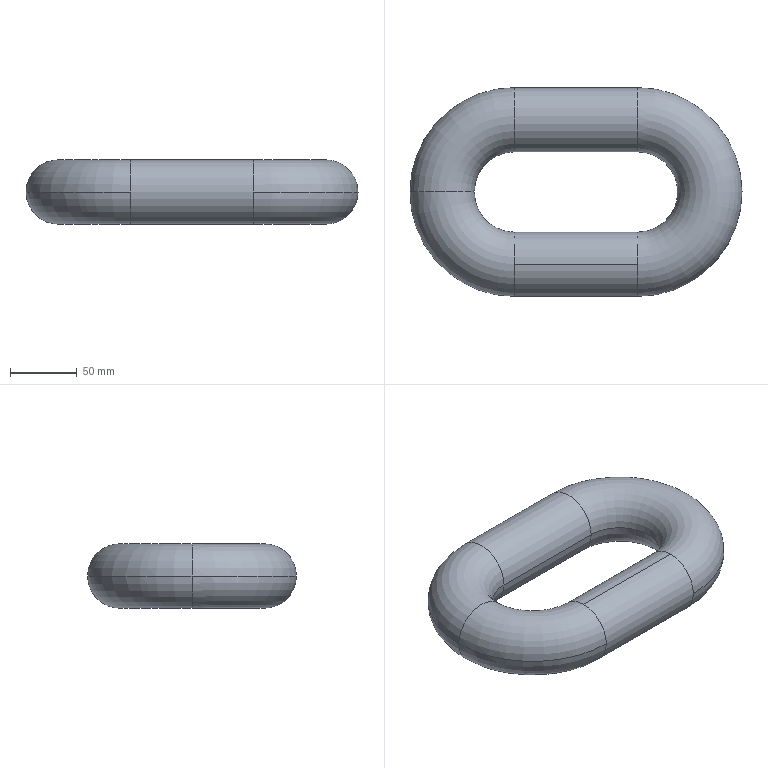Part | SolidWorks | features Sweep 1 | 1 solid | 10 faces | box 248 x 156 x 48 mm | volume 946927 mm3 | torus 6 | cylinder 4 | commonest cylinder face diameters 48 x4
STEP:
#1=CARTESIAN_POINT('',(-30.,0.,0.));
#2=VERTEX_POINT('',#1);
#3=CARTESIAN_POINT('',(-78.,0.,0.));
#4=VERTEX_POINT('',#3);
#5=CARTESIAN_POINT('',(-54.,0.,0.));
#6=DIRECTION('',(0.,1.,0.));
#7=DIRECTION('',(0.,0.,1.));
#8=AXIS2_PLACEMENT_3D('',#5,#6,#7);
#9=CIRCLE('',#8,24.);
#10=EDGE_CURVE('',#2,#4,#9,.T.);
#11=ORIENTED_EDGE('',*,*,#10,.T.);
#12=CARTESIAN_POINT('',(0.,78.,0.));
#13=VERTEX_POINT('',#12);
#14=CARTESIAN_POINT('',(0.,0.,0.));
#15=DIRECTION('',(0.,0.,-1.));
#16=DIRECTION('',(-1.,0.,0.));
#17=AXIS2_PLACEMENT_3D('',#14,#15,#16);
#18=CIRCLE('',#17,78.);
#19=EDGE_CURVE('',#4,#13,#18,.T.);
#20=ORIENTED_EDGE('',*,*,#19,.T.);
#21=CARTESIAN_POINT('',(0.,30.,0.));
#22=VERTEX_POINT('',#21);
#23=CARTESIAN_POINT('',(0.,54.,0.));
#24=DIRECTION('',(1.,0.,0.));
#25=DIRECTION('',(0.,0.,1.));
#26=AXIS2_PLACEMENT_3D('',#23,#24,#25);
#27=CIRCLE('',#26,24.);
#28=EDGE_CURVE('',#22,#13,#27,.T.);
#29=ORIENTED_EDGE('',*,*,#28,.F.);
#30=CARTESIAN_POINT('',(0.,0.,0.));
#31=DIRECTION('',(0.,0.,-1.));
#32=DIRECTION('',(-1.,0.,0.));
#33=AXIS2_PLACEMENT_3D('',#30,#31,#32);
#34=CIRCLE('',#33,30.);
#35=EDGE_CURVE('',#2,#22,#34,.T.);
#36=ORIENTED_EDGE('',*,*,#35,.F.);
#37=EDGE_LOOP('',(#11,#20,#29,#36));
#38=FACE_OUTER_BOUND('',#37,.T.);
#39=CARTESIAN_POINT('',(0.,0.,0.));
#40=DIRECTION('',(0.,0.,-1.));
#41=DIRECTION('',(-1.,0.,0.));
#42=AXIS2_PLACEMENT_3D('',#39,#40,#41);
#43=TOROIDAL_SURFACE('',#42,54.,24.);
#44=ADVANCED_FACE('',(#38),#43,.T.);
#45=CARTESIAN_POINT('',(92.,30.,0.));
#46=VERTEX_POINT('',#45);
#47=CARTESIAN_POINT('',(92.,78.,0.));
#48=VERTEX_POINT('',#47);
#49=CARTESIAN_POINT('',(92.,54.,0.));
#50=DIRECTION('',(1.,0.,0.));
#51=DIRECTION('',(0.,0.,1.));
#52=AXIS2_PLACEMENT_3D('',#49,#50,#51);
#53=CIRCLE('',#52,24.);
#54=EDGE_CURVE('',#46,#48,#53,.T.);
#55=ORIENTED_EDGE('',*,*,#54,.T.);
#56=CARTESIAN_POINT('',(92.,-78.,0.));
#57=VERTEX_POINT('',#56);
#58=CARTESIAN_POINT('',(92.,0.,0.));
#59=DIRECTION('',(0.,0.,-1.));
#60=DIRECTION('',(-1.,0.,0.));
#61=AXIS2_PLACEMENT_3D('',#58,#59,#60);
#62=CIRCLE('',#61,78.);
#63=EDGE_CURVE('',#48,#57,#62,.T.);
#64=ORIENTED_EDGE('',*,*,#63,.T.);
#65=CARTESIAN_POINT('',(92.,-54.,-24.));
#66=VERTEX_POINT('',#65);
#67=CARTESIAN_POINT('',(92.,-54.,0.));
#68=DIRECTION('',(-1.,0.,0.));
#69=DIRECTION('',(0.,0.,1.));
#70=AXIS2_PLACEMENT_3D('',#67,#68,#69);
#71=CIRCLE('',#70,24.);
#72=EDGE_CURVE('',#66,#57,#71,.T.);
#73=ORIENTED_EDGE('',*,*,#72,.F.);
#74=CARTESIAN_POINT('',(92.,-30.,0.));
#75=VERTEX_POINT('',#74);
#76=CARTESIAN_POINT('',(92.,-54.,0.));
#77=DIRECTION('',(-1.,0.,0.));
#78=DIRECTION('',(0.,0.,1.));
#79=AXIS2_PLACEMENT_3D('',#76,#77,#78);
#80=CIRCLE('',#79,24.);
#81=EDGE_CURVE('',#75,#66,#80,.T.);
#82=ORIENTED_EDGE('',*,*,#81,.F.);
#83=CARTESIAN_POINT('',(92.,0.,0.));
#84=DIRECTION('',(0.,0.,-1.));
#85=DIRECTION('',(-1.,0.,0.));
#86=AXIS2_PLACEMENT_3D('',#83,#84,#85);
#87=CIRCLE('',#86,30.);
#88=EDGE_CURVE('',#46,#75,#87,.T.);
#89=ORIENTED_EDGE('',*,*,#88,.F.);
#90=EDGE_LOOP('',(#55,#64,#73,#82,#89));
#91=FACE_OUTER_BOUND('',#90,.T.);
#92=CARTESIAN_POINT('',(92.,0.,0.));
#93=DIRECTION('',(0.,0.,-1.));
#94=DIRECTION('',(-1.,0.,0.));
#95=AXIS2_PLACEMENT_3D('',#92,#93,#94);
#96=TOROIDAL_SURFACE('',#95,54.,24.);
#97=ADVANCED_FACE('',(#91),#96,.T.);
#98=CARTESIAN_POINT('',(0.,-54.,-24.));
#99=VERTEX_POINT('',#98);
#100=CARTESIAN_POINT('',(0.,-78.,0.));
#101=VERTEX_POINT('',#100);
#102=CARTESIAN_POINT('',(0.,-54.,0.));
#103=DIRECTION('',(-1.,0.,0.));
#104=DIRECTION('',(0.,0.,1.));
#105=AXIS2_PLACEMENT_3D('',#102,#103,#104);
#106=CIRCLE('',#105,24.);
#107=EDGE_CURVE('',#99,#101,#106,.T.);
#108=ORIENTED_EDGE('',*,*,#107,.T.);
#109=CARTESIAN_POINT('',(0.,0.,0.));
#110=DIRECTION('',(0.,0.,-1.));
#111=DIRECTION('',(-1.,0.,0.));
#112=AXIS2_PLACEMENT_3D('',#109,#110,#111);
#113=CIRCLE('',#112,78.);
#114=EDGE_CURVE('',#101,#4,#113,.T.);
#115=ORIENTED_EDGE('',*,*,#114,.T.);
#116=ORIENTED_EDGE('',*,*,#10,.F.);
#117=CARTESIAN_POINT('',(0.,-30.,0.));
#118=VERTEX_POINT('',#117);
#119=CARTESIAN_POINT('',(0.,0.,0.));
#120=DIRECTION('',(0.,0.,-1.));
#121=DIRECTION('',(-1.,0.,0.));
#122=AXIS2_PLACEMENT_3D('',#119,#120,#121);
#123=CIRCLE('',#122,30.);
#124=EDGE_CURVE('',#118,#2,#123,.T.);
#125=ORIENTED_EDGE('',*,*,#124,.F.);
#126=CARTESIAN_POINT('',(0.,-54.,0.));
#127=DIRECTION('',(-1.,0.,0.));
#128=DIRECTION('',(0.,0.,1.));
#129=AXIS2_PLACEMENT_3D('',#126,#127,#128);
#130=CIRCLE('',#129,24.);
#131=EDGE_CURVE('',#118,#99,#130,.T.);
#132=ORIENTED_EDGE('',*,*,#131,.T.);
#133=EDGE_LOOP('',(#108,#115,#116,#125,#132));
#134=FACE_OUTER_BOUND('',#133,.T.);
#135=CARTESIAN_POINT('',(0.,0.,0.));
#136=DIRECTION('',(0.,0.,-1.));
#137=DIRECTION('',(-1.,0.,0.));
#138=AXIS2_PLACEMENT_3D('',#135,#136,#137);
#139=TOROIDAL_SURFACE('',#138,54.,24.);
#140=ADVANCED_FACE('',(#134),#139,.T.);
#141=CARTESIAN_POINT('',(0.,54.,0.));
#142=DIRECTION('',(1.,0.,0.));
#143=DIRECTION('',(0.,0.,1.));
#144=AXIS2_PLACEMENT_3D('',#141,#142,#143);
#145=CIRCLE('',#144,24.);
#146=EDGE_CURVE('',#13,#22,#145,.T.);
#147=ORIENTED_EDGE('',*,*,#146,.T.);
#148=CARTESIAN_POINT('',(0.,30.,0.));
#149=DIRECTION('',(1.,0.,0.));
#150=VECTOR('',#149,1000.);
#151=LINE('',#148,#150);
#152=EDGE_CURVE('',#22,#46,#151,.T.);
#153=ORIENTED_EDGE('',*,*,#152,.T.);
#154=CARTESIAN_POINT('',(92.,54.,0.));
#155=DIRECTION('',(1.,0.,0.));
#156=DIRECTION('',(0.,0.,1.));
#157=AXIS2_PLACEMENT_3D('',#154,#155,#156);
#158=CIRCLE('',#157,24.);
#159=EDGE_CURVE('',#48,#46,#158,.T.);
#160=ORIENTED_EDGE('',*,*,#159,.F.);
#161=CARTESIAN_POINT('',(0.,78.,0.));
#162=DIRECTION('',(1.,0.,0.));
#163=VECTOR('',#162,1000.);
#164=LINE('',#161,#163);
#165=EDGE_CURVE('',#13,#48,#164,.T.);
#166=ORIENTED_EDGE('',*,*,#165,.F.);
#167=EDGE_LOOP('',(#147,#153,#160,#166));
#168=FACE_OUTER_BOUND('',#167,.T.);
#169=CARTESIAN_POINT('',(0.,54.,0.));
#170=DIRECTION('',(1.,0.,0.));
#171=DIRECTION('',(0.,1.,0.));
#172=AXIS2_PLACEMENT_3D('',#169,#170,#171);
#173=CYLINDRICAL_SURFACE('',#172,24.);
#174=ADVANCED_FACE('',(#168),#173,.T.);
#175=CARTESIAN_POINT('',(92.,-54.,24.));
#176=VERTEX_POINT('',#175);
#177=CARTESIAN_POINT('',(92.,-54.,0.));
#178=DIRECTION('',(-1.,0.,0.));
#179=DIRECTION('',(0.,0.,1.));
#180=AXIS2_PLACEMENT_3D('',#177,#178,#179);
#181=CIRCLE('',#180,24.);
#182=EDGE_CURVE('',#176,#75,#181,.T.);
#183=ORIENTED_EDGE('',*,*,#182,.T.);
#184=ORIENTED_EDGE('',*,*,#81,.T.);
#185=CARTESIAN_POINT('',(92.,-54.,-24.));
#186=DIRECTION('',(-1.,0.,0.));
#187=VECTOR('',#186,1000.);
#188=LINE('',#185,#187);
#189=EDGE_CURVE('',#66,#99,#188,.T.);
#190=ORIENTED_EDGE('',*,*,#189,.T.);
#191=ORIENTED_EDGE('',*,*,#131,.F.);
#192=CARTESIAN_POINT('',(0.,-54.,24.));
#193=VERTEX_POINT('',#192);
#194=CARTESIAN_POINT('',(0.,-54.,0.));
#195=DIRECTION('',(-1.,0.,0.));
#196=DIRECTION('',(0.,0.,1.));
#197=AXIS2_PLACEMENT_3D('',#194,#195,#196);
#198=CIRCLE('',#197,24.);
#199=EDGE_CURVE('',#193,#118,#198,.T.);
#200=ORIENTED_EDGE('',*,*,#199,.F.);
#201=CARTESIAN_POINT('',(92.,-54.,24.));
#202=DIRECTION('',(-1.,0.,0.));
#203=VECTOR('',#202,1000.);
#204=LINE('',#201,#203);
#205=EDGE_CURVE('',#176,#193,#204,.T.);
#206=ORIENTED_EDGE('',*,*,#205,.F.);
#207=EDGE_LOOP('',(#183,#184,#190,#191,#200,#206));
#208=FACE_OUTER_BOUND('',#207,.T.);
#209=CARTESIAN_POINT('',(92.,-54.,0.));
#210=DIRECTION('',(-1.,0.,0.));
#211=DIRECTION('',(0.,0.,1.));
#212=AXIS2_PLACEMENT_3D('',#209,#210,#211);
#213=CYLINDRICAL_SURFACE('',#212,24.);
#214=ADVANCED_FACE('',(#208),#213,.T.);
#215=ORIENTED_EDGE('',*,*,#114,.F.);
#216=CARTESIAN_POINT('',(0.,-54.,0.));
#217=DIRECTION('',(-1.,0.,0.));
#218=DIRECTION('',(0.,0.,1.));
#219=AXIS2_PLACEMENT_3D('',#216,#217,#218);
#220=CIRCLE('',#219,24.);
#221=EDGE_CURVE('',#101,#193,#220,.T.);
#222=ORIENTED_EDGE('',*,*,#221,.T.);
#223=ORIENTED_EDGE('',*,*,#199,.T.);
#224=ORIENTED_EDGE('',*,*,#124,.T.);
#225=CARTESIAN_POINT('',(-54.,0.,0.));
#226=DIRECTION('',(0.,1.,0.));
#227=DIRECTION('',(0.,0.,1.));
#228=AXIS2_PLACEMENT_3D('',#225,#226,#227);
#229=CIRCLE('',#228,24.);
#230=EDGE_CURVE('',#4,#2,#229,.T.);
#231=ORIENTED_EDGE('',*,*,#230,.F.);
#232=EDGE_LOOP('',(#215,#222,#223,#224,#231));
#233=FACE_OUTER_BOUND('',#232,.T.);
#234=CARTESIAN_POINT('',(0.,0.,0.));
#235=DIRECTION('',(0.,0.,-1.));
#236=DIRECTION('',(-1.,0.,0.));
#237=AXIS2_PLACEMENT_3D('',#234,#235,#236);
#238=TOROIDAL_SURFACE('',#237,54.,24.);
#239=ADVANCED_FACE('',(#233),#238,.T.);
#240=ORIENTED_EDGE('',*,*,#189,.F.);
#241=ORIENTED_EDGE('',*,*,#72,.T.);
#242=CARTESIAN_POINT('',(92.,-54.,0.));
#243=DIRECTION('',(-1.,0.,0.));
#244=DIRECTION('',(0.,0.,1.));
#245=AXIS2_PLACEMENT_3D('',#242,#243,#244);
#246=CIRCLE('',#245,24.);
#247=EDGE_CURVE('',#57,#176,#246,.T.);
#248=ORIENTED_EDGE('',*,*,#247,.T.);
#249=ORIENTED_EDGE('',*,*,#205,.T.);
#250=ORIENTED_EDGE('',*,*,#221,.F.);
#251=ORIENTED_EDGE('',*,*,#107,.F.);
#252=EDGE_LOOP('',(#240,#241,#248,#249,#250,#251));
#253=FACE_OUTER_BOUND('',#252,.T.);
#254=CARTESIAN_POINT('',(92.,-54.,0.));
#255=DIRECTION('',(-1.,0.,0.));
#256=DIRECTION('',(0.,0.,1.));
#257=AXIS2_PLACEMENT_3D('',#254,#255,#256);
#258=CYLINDRICAL_SURFACE('',#257,24.);
#259=ADVANCED_FACE('',(#253),#258,.T.);
#260=ORIENTED_EDGE('',*,*,#63,.F.);
#261=ORIENTED_EDGE('',*,*,#159,.T.);
#262=ORIENTED_EDGE('',*,*,#88,.T.);
#263=ORIENTED_EDGE('',*,*,#182,.F.);
#264=ORIENTED_EDGE('',*,*,#247,.F.);
#265=EDGE_LOOP('',(#260,#261,#262,#263,#264));
#266=FACE_OUTER_BOUND('',#265,.T.);
#267=CARTESIAN_POINT('',(92.,0.,0.));
#268=DIRECTION('',(0.,0.,-1.));
#269=DIRECTION('',(-1.,0.,0.));
#270=AXIS2_PLACEMENT_3D('',#267,#268,#269);
#271=TOROIDAL_SURFACE('',#270,54.,24.);
#272=ADVANCED_FACE('',(#266),#271,.T.);
#273=ORIENTED_EDGE('',*,*,#152,.F.);
#274=ORIENTED_EDGE('',*,*,#28,.T.);
#275=ORIENTED_EDGE('',*,*,#165,.T.);
#276=ORIENTED_EDGE('',*,*,#54,.F.);
#277=EDGE_LOOP('',(#273,#274,#275,#276));
#278=FACE_OUTER_BOUND('',#277,.T.);
#279=CARTESIAN_POINT('',(0.,54.,0.));
#280=DIRECTION('',(1.,0.,0.));
#281=DIRECTION('',(0.,1.,0.));
#282=AXIS2_PLACEMENT_3D('',#279,#280,#281);
#283=CYLINDRICAL_SURFACE('',#282,24.);
#284=ADVANCED_FACE('',(#278),#283,.T.);
#285=ORIENTED_EDGE('',*,*,#19,.F.);
#286=ORIENTED_EDGE('',*,*,#230,.T.);
#287=ORIENTED_EDGE('',*,*,#35,.T.);
#288=ORIENTED_EDGE('',*,*,#146,.F.);
#289=EDGE_LOOP('',(#285,#286,#287,#288));
#290=FACE_OUTER_BOUND('',#289,.T.);
#291=CARTESIAN_POINT('',(0.,0.,0.));
#292=DIRECTION('',(0.,0.,-1.));
#293=DIRECTION('',(-1.,0.,0.));
#294=AXIS2_PLACEMENT_3D('',#291,#292,#293);
#295=TOROIDAL_SURFACE('',#294,54.,24.);
#296=ADVANCED_FACE('',(#290),#295,.T.);
#297=CLOSED_SHELL('',(#44,#97,#140,#174,#214,#239,#259,#272,#284,#296));
#298=MANIFOLD_SOLID_BREP('',#297);
#299=CARTESIAN_POINT('',(0.,0.,0.));
#300=DIRECTION('',(0.,0.,1.));
#301=DIRECTION('',(1.,0.,0.));
#302=AXIS2_PLACEMENT_3D('',#299,#300,#301);
#303=(LENGTH_UNIT()NAMED_UNIT(*)SI_UNIT(.MILLI.,.METRE.));
#304=UNCERTAINTY_MEASURE_WITH_UNIT(LENGTH_MEASURE(0.00001),#303,'','');
#305=(NAMED_UNIT(*)PLANE_ANGLE_UNIT()SI_UNIT($,.RADIAN.));
#306=(NAMED_UNIT(*)SI_UNIT($,.STERADIAN.)SOLID_ANGLE_UNIT());
#307=(GEOMETRIC_REPRESENTATION_CONTEXT(3)GLOBAL_UNCERTAINTY_ASSIGNED_CONTEXT((#304))GLOBAL_UNIT_ASSIGNED_CONTEXT((#303,#305,#306))REPRESENTATION_CONTEXT('',''));
#308=ADVANCED_BREP_SHAPE_REPRESENTATION('',(#298,#302),#307);